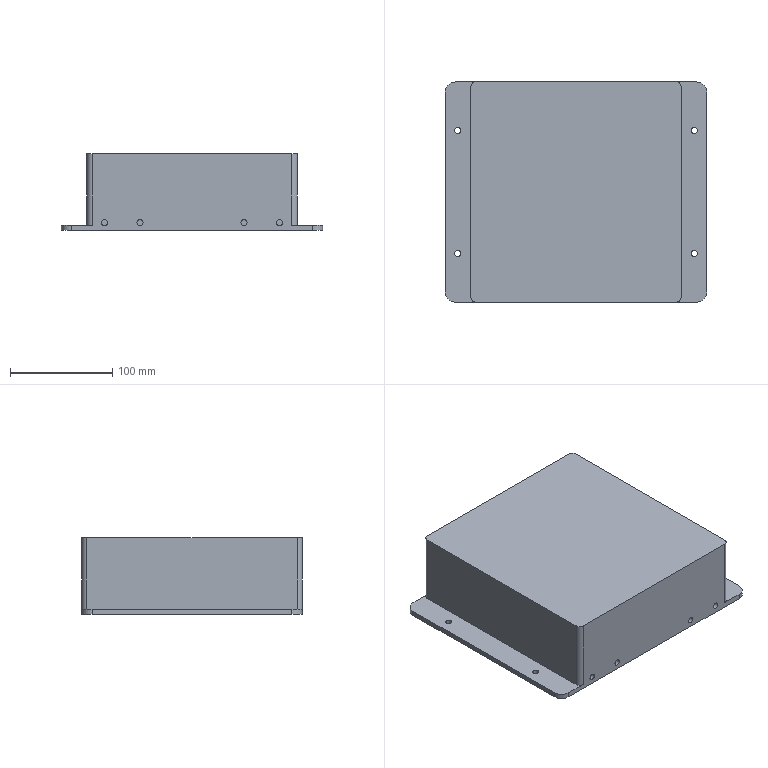NC program | NX | posted with a generic post | part box 255 x 215 x 75 mm
Lines 1 to 26 of 12583:
N10 G17 G21 G94 G90
(FLOOR_WALL , TOOL : D80)
N12 T19 M6
N14 G54
N16 G17 G0 G90 X-175.5 Y112.497 B0. C0. S6500 M3
N18 G43 Z30. H19
N20 Z3.
N22 G94 G1 Z0. F1500.
N24 X-172.5
N26 X172.5
N28 Y64.248
N30 X-172.5
N32 Y15.999
N34 X172.5
N36 Y-32.251
N38 X-172.5
N40 Y-80.5
N42 X172.5
N44 X175.5
N46 Z3.
N48 G0 Z30.
N50 M5